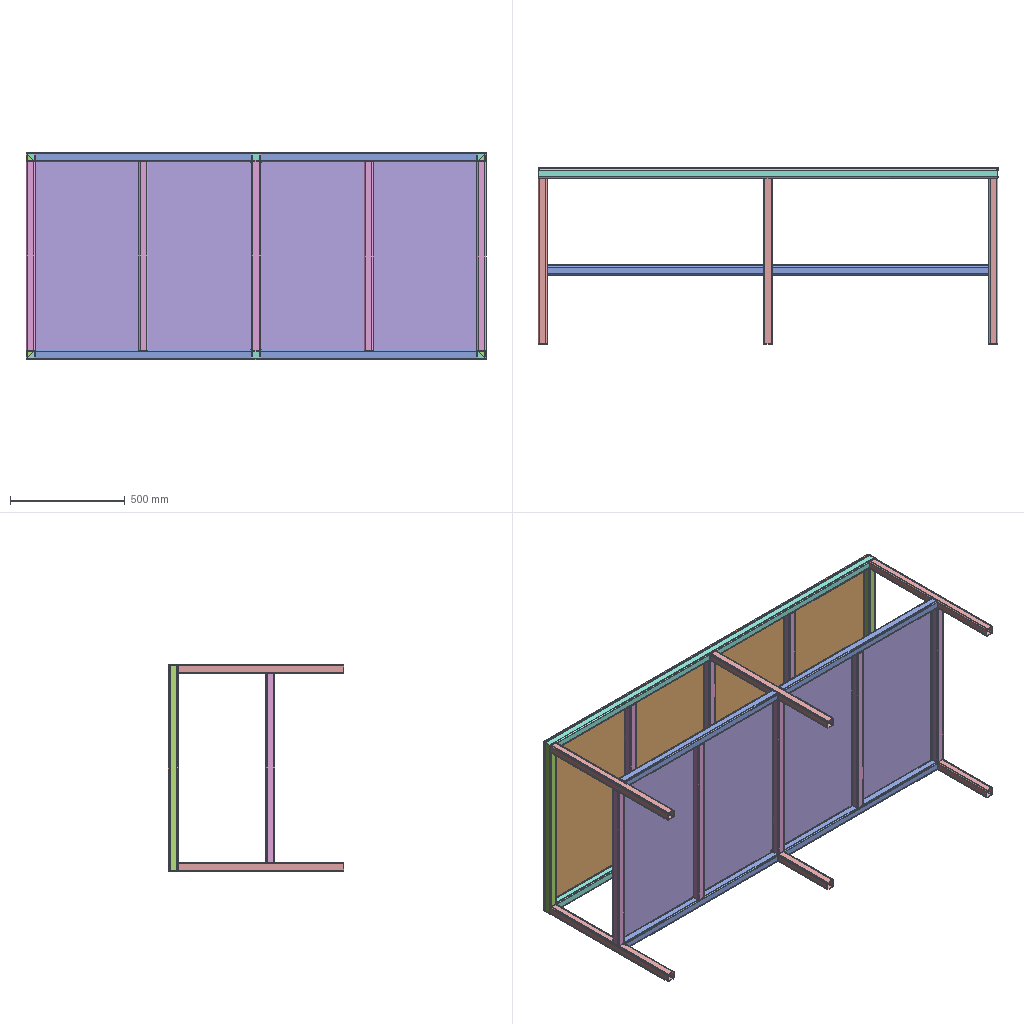Assembly | SolidWorks | 8 different items | 26 placed | box 2000 x 765 x 900 mm
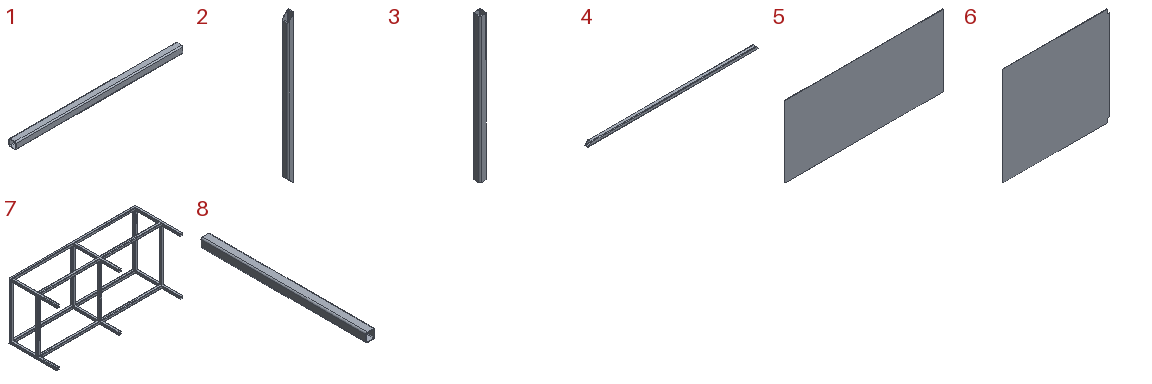Parts list (item | quantity | size | volume | features):
1 | x4 | 940 x 40 x 40 mm | 417990 mm3 | features SavedExtBody 1
2 | x2 | 40 x 40 x 900 mm | 382416 mm3 | features SavedExtBody 1
3 | x8 | 40 x 40 x 820 mm | 364629 mm3 | features SavedExtBody 1
4 | x2 | 2000 x 40 x 40 mm | 871553 mm3 | features SavedExtBody 1
5 | x1 | 2000 x 5 x 900 mm | 8999845 mm3 | features Extrusion 1, Fillet 1
6 | x2 | 956 x 3 x 885 mm | 2533644 mm3 | features Extrusion 1
7 | x1 | 2000 x 760 x 900 mm | 7559385 mm3 | features 3DProfileFeature 1, CosmeticWeldCutList 1, WeldMemberFeat 1, WeldmentFeature 1
8 | x6 | 40 x 720 x 40 mm | 320162 mm3 | features SavedExtBody 1
Mates (type | each side: item.copy, entity, surface, feature):
Coincident | 2.1 face plane Base part-V8 vertical lathe tool rack-1 | 4.1 face plane Base part-V8 vertical lathe tool rack-1 | 2 times
Coincident | 2.1 edge | 4.1 edge
Coincident | 8.1 face plane Base part-V8 vertical lathe tool rack-1 | 4.1 face plane Base part-V8 vertical lathe tool rack-1 | 2 times
Coincident | 8.1 face plane Base part-V8 vertical lathe tool rack-1 | 2.1 face plane Base part-V8 vertical lathe tool rack-1
Coincident | 8.1 face plane Base part-V8 vertical lathe tool rack-1 | 3.1 face plane Base part-V8 vertical lathe tool rack-1 | 2 times
Coincident | 1.1 face plane Base part-V8 vertical lathe tool rack-1 | 3.1 face plane Base part-V8 vertical lathe tool rack-1
Coincident | 8.1 face plane Base part-V8 vertical lathe tool rack-1 | 1.1 face plane Base part-V8 vertical lathe tool rack-1 | 2 times
DistanceDim | 3.1 face plane Base part-V8 vertical lathe tool rack-1 | 8.1 face plane Base part-V8 vertical lathe tool rack-1
Coincident | 2.1 face plane Base part-V8 vertical lathe tool rack-1 | 5.1 face plane Boss-Extrude1
Coincident | 4.1 face plane Base part-V8 vertical lathe tool rack-1 | 5.1 face plane Boss-Extrude1
Coincident | 8.1 face plane Base part-V8 vertical lathe tool rack-1 | 5.1 face plane Boss-Extrude1
Coincident | 3.2 face plane Base part-V8 vertical lathe tool rack-1 | 6.1 face plane Boss-Extrude1
DistanceDim | 6.1 face plane Boss-Extrude1 | 3.2 face plane Base part-V8 vertical lathe tool rack-1
DistanceDim | 6.1 face plane Boss-Extrude1 | 8.2 face plane Base part-V8 vertical lathe tool rack-1